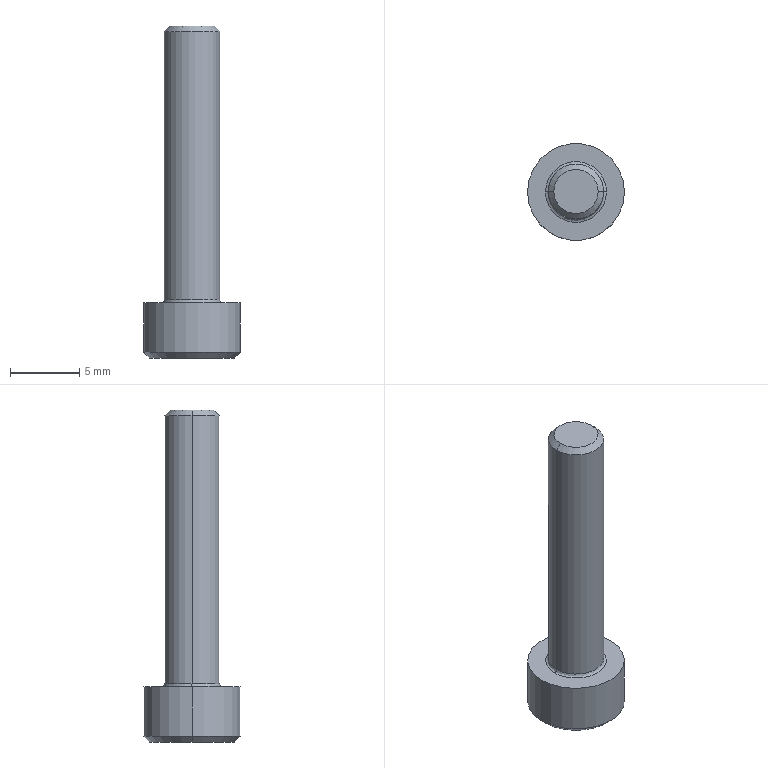Part | STEP file | 1 solid | 20 faces | box 7 x 7 x 24 mm | volume 380.939 mm3 | plane 10 | cone 4 | cylinder 4 | spline 2 | commonest cylinder face diameters 4 x2 7 x2